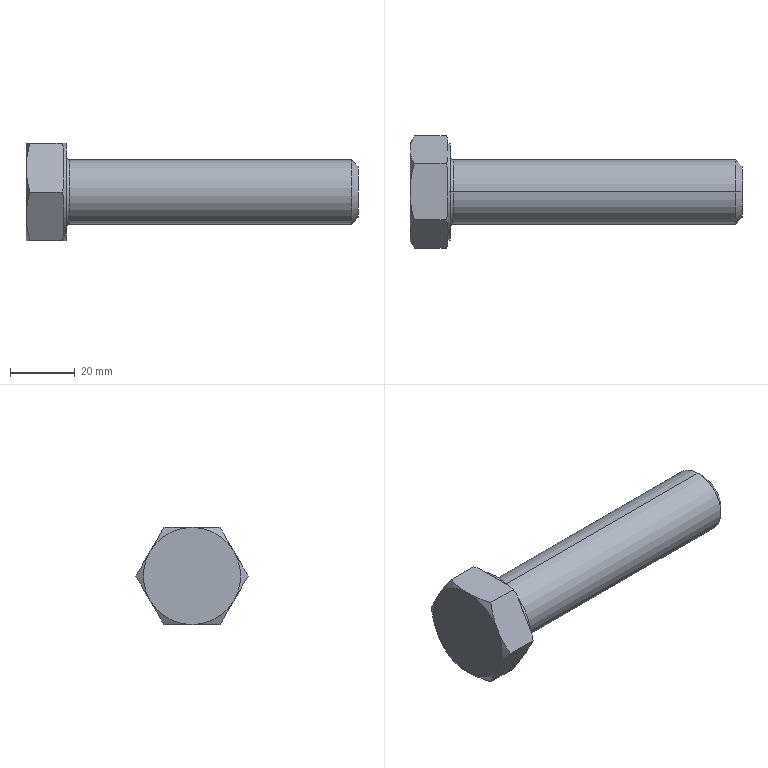Part | SolidWorks | features RevCut 4, Chamfer 1, Extrusion 1, Fillet 1, LPattern 1, Revolution 1 | 1 solid | 35 faces | box 102.5 x 34.641 x 30 mm | volume 37820 mm3 | plane 15 | cone 14 | cylinder 4 | torus 2 | commonest cylinder face diameters 20 x2 30 x2
STEP:
#1=CARTESIAN_POINT('',(13.3,0.,10.));
#2=VERTEX_POINT('',#1);
#3=CARTESIAN_POINT('',(13.3,0.,-10.));
#4=VERTEX_POINT('',#3);
#5=CARTESIAN_POINT('',(13.3,0.,0.));
#6=DIRECTION('',(1.,0.,0.));
#7=DIRECTION('',(0.,0.,-1.));
#8=AXIS2_PLACEMENT_3D('',#5,#6,#7);
#9=CIRCLE('',#8,10.);
#10=EDGE_CURVE('',#2,#4,#9,.T.);
#11=ORIENTED_EDGE('',*,*,#10,.F.);
#12=CARTESIAN_POINT('',(12.5,0.,10.8));
#13=VERTEX_POINT('',#12);
#14=CARTESIAN_POINT('',(13.3,0.,10.8));
#15=DIRECTION('',(0.,1.,0.));
#16=DIRECTION('',(0.,0.,1.));
#17=AXIS2_PLACEMENT_3D('',#14,#15,#16);
#18=CIRCLE('',#17,0.8);
#19=EDGE_CURVE('',#2,#13,#18,.T.);
#20=ORIENTED_EDGE('',*,*,#19,.T.);
#21=CARTESIAN_POINT('',(12.5,0.,-10.8));
#22=VERTEX_POINT('',#21);
#23=CARTESIAN_POINT('',(12.5,0.,0.));
#24=DIRECTION('',(-1.,0.,0.));
#25=DIRECTION('',(0.,0.,-1.));
#26=AXIS2_PLACEMENT_3D('',#23,#24,#25);
#27=CIRCLE('',#26,10.8);
#28=EDGE_CURVE('',#22,#13,#27,.T.);
#29=ORIENTED_EDGE('',*,*,#28,.F.);
#30=CARTESIAN_POINT('',(13.3,0.,-10.8));
#31=DIRECTION('',(0.,-1.,0.));
#32=DIRECTION('',(0.,0.,-1.));
#33=AXIS2_PLACEMENT_3D('',#30,#31,#32);
#34=CIRCLE('',#33,0.8);
#35=EDGE_CURVE('',#4,#22,#34,.T.);
#36=ORIENTED_EDGE('',*,*,#35,.F.);
#37=EDGE_LOOP('',(#11,#20,#29,#36));
#38=FACE_OUTER_BOUND('',#37,.T.);
#39=CARTESIAN_POINT('',(13.3,0.,0.));
#40=DIRECTION('',(1.,0.,0.));
#41=DIRECTION('',(0.,0.,-1.));
#42=AXIS2_PLACEMENT_3D('',#39,#40,#41);
#43=TOROIDAL_SURFACE('',#42,10.8,0.8);
#44=ADVANCED_FACE('',(#38),#43,.F.);
#45=CARTESIAN_POINT('',(102.5,0.,-8.));
#46=VERTEX_POINT('',#45);
#47=CARTESIAN_POINT('',(102.5,0.,8.));
#48=VERTEX_POINT('',#47);
#49=CARTESIAN_POINT('',(102.5,0.,0.));
#50=DIRECTION('',(1.,0.,0.));
#51=DIRECTION('',(0.,0.,1.));
#52=AXIS2_PLACEMENT_3D('',#49,#50,#51);
#53=CIRCLE('',#52,8.);
#54=EDGE_CURVE('',#46,#48,#53,.T.);
#55=ORIENTED_EDGE('',*,*,#54,.F.);
#56=CARTESIAN_POINT('',(100.5,0.,-10.));
#57=VERTEX_POINT('',#56);
#58=CARTESIAN_POINT('',(100.5,0.,-10.));
#59=DIRECTION('',(-0.7071,0.,-0.7071));
#60=VECTOR('',#59,1000.);
#61=LINE('',#58,#60);
#62=EDGE_CURVE('',#46,#57,#61,.T.);
#63=ORIENTED_EDGE('',*,*,#62,.T.);
#64=CARTESIAN_POINT('',(100.5,0.,10.));
#65=VERTEX_POINT('',#64);
#66=CARTESIAN_POINT('',(100.5,0.,0.));
#67=DIRECTION('',(-1.,0.,0.));
#68=DIRECTION('',(0.,0.,1.));
#69=AXIS2_PLACEMENT_3D('',#66,#67,#68);
#70=CIRCLE('',#69,10.);
#71=EDGE_CURVE('',#65,#57,#70,.T.);
#72=ORIENTED_EDGE('',*,*,#71,.F.);
#73=CARTESIAN_POINT('',(100.5,0.,10.));
#74=DIRECTION('',(-0.7071,0.,0.7071));
#75=VECTOR('',#74,1000.);
#76=LINE('',#73,#75);
#77=EDGE_CURVE('',#48,#65,#76,.T.);
#78=ORIENTED_EDGE('',*,*,#77,.F.);
#79=EDGE_LOOP('',(#55,#63,#72,#78));
#80=FACE_OUTER_BOUND('',#79,.T.);
#81=CARTESIAN_POINT('',(100.5,0.,0.));
#82=DIRECTION('',(-1.,0.,0.));
#83=DIRECTION('',(0.,0.,1.));
#84=AXIS2_PLACEMENT_3D('',#81,#82,#83);
#85=CONICAL_SURFACE('',#84,10.,0.7854);
#86=ADVANCED_FACE('',(#80),#85,.T.);
#87=ORIENTED_EDGE('',*,*,#71,.T.);
#88=CARTESIAN_POINT('',(0.,0.,-10.));
#89=DIRECTION('',(-1.,0.,0.));
#90=VECTOR('',#89,1000.);
#91=LINE('',#88,#90);
#92=EDGE_CURVE('',#57,#4,#91,.T.);
#93=ORIENTED_EDGE('',*,*,#92,.T.);
#94=CARTESIAN_POINT('',(13.3,0.,0.));
#95=DIRECTION('',(1.,0.,0.));
#96=DIRECTION('',(0.,0.,-1.));
#97=AXIS2_PLACEMENT_3D('',#94,#95,#96);
#98=CIRCLE('',#97,10.);
#99=EDGE_CURVE('',#4,#2,#98,.T.);
#100=ORIENTED_EDGE('',*,*,#99,.T.);
#101=CARTESIAN_POINT('',(0.,0.,10.));
#102=DIRECTION('',(-1.,0.,0.));
#103=VECTOR('',#102,1000.);
#104=LINE('',#101,#103);
#105=EDGE_CURVE('',#65,#2,#104,.T.);
#106=ORIENTED_EDGE('',*,*,#105,.F.);
#107=EDGE_LOOP('',(#87,#93,#100,#106));
#108=FACE_OUTER_BOUND('',#107,.T.);
#109=CARTESIAN_POINT('',(0.,0.,0.));
#110=DIRECTION('',(-1.,0.,0.));
#111=DIRECTION('',(0.,0.,1.));
#112=AXIS2_PLACEMENT_3D('',#109,#110,#111);
#113=CYLINDRICAL_SURFACE('',#112,10.);
#114=ADVANCED_FACE('',(#108),#113,.T.);
#115=CARTESIAN_POINT('',(12.5,0.,-15.));
#116=VERTEX_POINT('',#115);
#117=CARTESIAN_POINT('',(12.5,0.,15.));
#118=VERTEX_POINT('',#117);
#119=CARTESIAN_POINT('',(12.5,0.,0.));
#120=DIRECTION('',(1.,0.,0.));
#121=DIRECTION('',(0.,0.,-1.));
#122=AXIS2_PLACEMENT_3D('',#119,#120,#121);
#123=CIRCLE('',#122,15.);
#124=EDGE_CURVE('',#116,#118,#123,.T.);
#125=ORIENTED_EDGE('',*,*,#124,.F.);
#126=CARTESIAN_POINT('',(11.7,0.,-15.));
#127=VERTEX_POINT('',#126);
#128=CARTESIAN_POINT('',(0.,0.,-15.));
#129=DIRECTION('',(-1.,0.,0.));
#130=VECTOR('',#129,1000.);
#131=LINE('',#128,#130);
#132=EDGE_CURVE('',#116,#127,#131,.T.);
#133=ORIENTED_EDGE('',*,*,#132,.T.);
#134=CARTESIAN_POINT('',(11.7,12.99,-7.5));
#135=VERTEX_POINT('',#134);
#136=CARTESIAN_POINT('',(11.7,0.,0.));
#137=DIRECTION('',(-1.,0.,0.));
#138=DIRECTION('',(0.,0.,1.));
#139=AXIS2_PLACEMENT_3D('',#136,#137,#138);
#140=CIRCLE('',#139,15.);
#141=EDGE_CURVE('',#135,#127,#140,.T.);
#142=ORIENTED_EDGE('',*,*,#141,.F.);
#143=CARTESIAN_POINT('',(11.7,12.99,7.5));
#144=VERTEX_POINT('',#143);
#145=CARTESIAN_POINT('',(11.7,0.,0.));
#146=DIRECTION('',(-1.,0.,0.));
#147=DIRECTION('',(0.,0.,1.));
#148=AXIS2_PLACEMENT_3D('',#145,#146,#147);
#149=CIRCLE('',#148,15.);
#150=EDGE_CURVE('',#144,#135,#149,.T.);
#151=ORIENTED_EDGE('',*,*,#150,.F.);
#152=CARTESIAN_POINT('',(11.7,0.,15.));
#153=VERTEX_POINT('',#152);
#154=CARTESIAN_POINT('',(11.7,0.,0.));
#155=DIRECTION('',(-1.,0.,0.));
#156=DIRECTION('',(0.,0.,1.));
#157=AXIS2_PLACEMENT_3D('',#154,#155,#156);
#158=CIRCLE('',#157,15.);
#159=EDGE_CURVE('',#153,#144,#158,.T.);
#160=ORIENTED_EDGE('',*,*,#159,.F.);
#161=CARTESIAN_POINT('',(0.,0.,15.));
#162=DIRECTION('',(-1.,0.,0.));
#163=VECTOR('',#162,1000.);
#164=LINE('',#161,#163);
#165=EDGE_CURVE('',#118,#153,#164,.T.);
#166=ORIENTED_EDGE('',*,*,#165,.F.);
#167=EDGE_LOOP('',(#125,#133,#142,#151,#160,#166));
#168=FACE_OUTER_BOUND('',#167,.T.);
#169=CARTESIAN_POINT('',(0.,0.,0.));
#170=DIRECTION('',(-1.,0.,0.));
#171=DIRECTION('',(0.,0.,1.));
#172=AXIS2_PLACEMENT_3D('',#169,#170,#171);
#173=CYLINDRICAL_SURFACE('',#172,15.);
#174=ADVANCED_FACE('',(#168),#173,.T.);
#175=CARTESIAN_POINT('',(11.7,9.693,-13.211));
#176=VERTEX_POINT('',#175);
#177=CARTESIAN_POINT('',(11.7,8.66,-15.));
#178=DIRECTION('',(0.,0.5,0.866));
#179=VECTOR('',#178,1000.);
#180=LINE('',#177,#179);
#181=EDGE_CURVE('',#176,#135,#180,.T.);
#182=ORIENTED_EDGE('',*,*,#181,.F.);
#183=CARTESIAN_POINT('',(11.16,8.66,-15.));
#184=VERTEX_POINT('',#183);
#185=CARTESIAN_POINT('',(11.16,8.66,-15.));
#186=CARTESIAN_POINT('',(11.358,9.003,-14.406));
#187=CARTESIAN_POINT('',(11.539,9.347,-13.81));
#188=CARTESIAN_POINT('',(11.7,9.693,-13.211));
#189=B_SPLINE_CURVE_WITH_KNOTS('',3,(#185,#186,#187,#188),.UNSPECIFIED.,.F.,.F.,(4,4),(0.000000238,0.002122),.UNSPECIFIED.);
#190=EDGE_CURVE('',#184,#176,#189,.T.);
#191=ORIENTED_EDGE('',*,*,#190,.F.);
#192=CARTESIAN_POINT('',(1.34,8.66,-15.));
#193=VERTEX_POINT('',#192);
#194=CARTESIAN_POINT('',(12.5,8.66,-15.));
#195=DIRECTION('',(-1.,0.,0.));
#196=VECTOR('',#195,1000.);
#197=LINE('',#194,#196);
#198=EDGE_CURVE('',#184,#193,#197,.T.);
#199=ORIENTED_EDGE('',*,*,#198,.T.);
#200=CARTESIAN_POINT('',(0.,12.99,-7.5));
#201=VERTEX_POINT('',#200);
#202=CARTESIAN_POINT('',(0.,12.99,-7.5));
#203=CARTESIAN_POINT('',(0.,12.623,-8.136));
#204=CARTESIAN_POINT('',(0.03167,12.254,-8.776));
#205=CARTESIAN_POINT('',(0.1542,11.524,-10.041));
#206=CARTESIAN_POINT('',(0.245,11.161,-10.669));
#207=CARTESIAN_POINT('',(0.595,10.079,-12.542));
#208=CARTESIAN_POINT('',(0.9318,9.367,-13.776));
#209=CARTESIAN_POINT('',(1.34,8.66,-15.));
#210=B_SPLINE_CURVE_WITH_KNOTS('',3,(#202,#203,#204,#205,#206,#207,#208,#209),.UNSPECIFIED.,.F.,.F.,(4,2,2,4),(0.008763,0.01095,0.01313,0.01749),.UNSPECIFIED.);
#211=EDGE_CURVE('',#201,#193,#210,.T.);
#212=ORIENTED_EDGE('',*,*,#211,.F.);
#213=CARTESIAN_POINT('',(1.34,17.321,0.));
#214=VERTEX_POINT('',#213);
#215=CARTESIAN_POINT('',(1.34,17.321,0.));
#216=CARTESIAN_POINT('',(0.9308,16.612,-1.227));
#217=CARTESIAN_POINT('',(0.5939,15.899,-2.463));
#218=CARTESIAN_POINT('',(0.1277,14.457,-4.96));
#219=CARTESIAN_POINT('',(0.,13.728,-6.222));
#220=CARTESIAN_POINT('',(0.,12.99,-7.5));
#221=B_SPLINE_CURVE_WITH_KNOTS('',3,(#215,#216,#217,#218,#219,#220),.UNSPECIFIED.,.F.,.F.,(4,2,4),(0.000000238,0.004382,0.008763),.UNSPECIFIED.);
#222=EDGE_CURVE('',#214,#201,#221,.T.);
#223=ORIENTED_EDGE('',*,*,#222,.F.);
#224=CARTESIAN_POINT('',(11.16,17.321,0.));
#225=VERTEX_POINT('',#224);
#226=CARTESIAN_POINT('',(12.5,17.321,0.));
#227=DIRECTION('',(-1.,0.,0.));
#228=VECTOR('',#227,1000.);
#229=LINE('',#226,#228);
#230=EDGE_CURVE('',#225,#214,#229,.T.);
#231=ORIENTED_EDGE('',*,*,#230,.F.);
#232=CARTESIAN_POINT('',(11.7,16.288,-1.789));
#233=VERTEX_POINT('',#232);
#234=CARTESIAN_POINT('',(11.7,16.288,-1.789));
#235=CARTESIAN_POINT('',(11.539,16.634,-1.19));
#236=CARTESIAN_POINT('',(11.358,16.978,-0.5937));
#237=CARTESIAN_POINT('',(11.16,17.321,0.));
#238=B_SPLINE_CURVE_WITH_KNOTS('',3,(#234,#235,#236,#237),.UNSPECIFIED.,.F.,.F.,(4,4),(0.01538,0.01749),.UNSPECIFIED.);
#239=EDGE_CURVE('',#233,#225,#238,.T.);
#240=ORIENTED_EDGE('',*,*,#239,.F.);
#241=CARTESIAN_POINT('',(11.7,8.66,-15.));
#242=DIRECTION('',(0.,0.5,0.866));
#243=VECTOR('',#242,1000.);
#244=LINE('',#241,#243);
#245=EDGE_CURVE('',#135,#233,#244,.T.);
#246=ORIENTED_EDGE('',*,*,#245,.F.);
#247=EDGE_LOOP('',(#182,#191,#199,#212,#223,#231,#240,#246));
#248=FACE_OUTER_BOUND('',#247,.T.);
#249=CARTESIAN_POINT('',(12.5,8.66,-15.));
#250=DIRECTION('',(0.,-0.866,0.5));
#251=DIRECTION('',(0.,-0.5,-0.866));
#252=AXIS2_PLACEMENT_3D('',#249,#250,#251);
#253=PLANE('',#252);
#254=ADVANCED_FACE('',(#248),#253,.F.);
#255=CARTESIAN_POINT('',(11.7,16.288,1.789));
#256=VERTEX_POINT('',#255);
#257=CARTESIAN_POINT('',(11.7,17.321,0.));
#258=DIRECTION('',(0.,-0.5,0.866));
#259=VECTOR('',#258,1000.);
#260=LINE('',#257,#259);
#261=EDGE_CURVE('',#256,#144,#260,.T.);
#262=ORIENTED_EDGE('',*,*,#261,.F.);
#263=CARTESIAN_POINT('',(11.16,17.321,0.));
#264=CARTESIAN_POINT('',(11.358,16.978,0.594));
#265=CARTESIAN_POINT('',(11.539,16.633,1.19));
#266=CARTESIAN_POINT('',(11.7,16.288,1.789));
#267=B_SPLINE_CURVE_WITH_KNOTS('',3,(#263,#264,#265,#266),.UNSPECIFIED.,.F.,.F.,(4,4),(0.000000238,0.002122),.UNSPECIFIED.);
#268=EDGE_CURVE('',#225,#256,#267,.T.);
#269=ORIENTED_EDGE('',*,*,#268,.F.);
#270=ORIENTED_EDGE('',*,*,#230,.T.);
#271=CARTESIAN_POINT('',(0.,12.99,7.5));
#272=VERTEX_POINT('',#271);
#273=CARTESIAN_POINT('',(0.,12.99,7.5));
#274=CARTESIAN_POINT('',(0.,13.358,6.864));
#275=CARTESIAN_POINT('',(0.03167,13.727,6.224));
#276=CARTESIAN_POINT('',(0.1542,14.457,4.959));
#277=CARTESIAN_POINT('',(0.245,14.82,4.331));
#278=CARTESIAN_POINT('',(0.595,15.901,2.458));
#279=CARTESIAN_POINT('',(0.9318,16.614,1.224));
#280=CARTESIAN_POINT('',(1.34,17.321,0.));
#281=B_SPLINE_CURVE_WITH_KNOTS('',3,(#273,#274,#275,#276,#277,#278,#279,#280),.UNSPECIFIED.,.F.,.F.,(4,2,2,4),(0.008763,0.01095,0.01313,0.01749),.UNSPECIFIED.);
#282=EDGE_CURVE('',#272,#214,#281,.T.);
#283=ORIENTED_EDGE('',*,*,#282,.F.);
#284=CARTESIAN_POINT('',(1.34,8.66,15.));
#285=VERTEX_POINT('',#284);
#286=CARTESIAN_POINT('',(1.34,8.66,15.));
#287=CARTESIAN_POINT('',(0.9308,9.369,13.773));
#288=CARTESIAN_POINT('',(0.5939,10.082,12.537));
#289=CARTESIAN_POINT('',(0.1277,11.524,10.04));
#290=CARTESIAN_POINT('',(0.,12.253,8.778));
#291=CARTESIAN_POINT('',(0.,12.99,7.5));
#292=B_SPLINE_CURVE_WITH_KNOTS('',3,(#286,#287,#288,#289,#290,#291),.UNSPECIFIED.,.F.,.F.,(4,2,4),(0.000000238,0.004382,0.008763),.UNSPECIFIED.);
#293=EDGE_CURVE('',#285,#272,#292,.T.);
#294=ORIENTED_EDGE('',*,*,#293,.F.);
#295=CARTESIAN_POINT('',(11.16,8.66,15.));
#296=VERTEX_POINT('',#295);
#297=CARTESIAN_POINT('',(12.5,8.66,15.));
#298=DIRECTION('',(-1.,0.,0.));
#299=VECTOR('',#298,1000.);
#300=LINE('',#297,#299);
#301=EDGE_CURVE('',#296,#285,#300,.T.);
#302=ORIENTED_EDGE('',*,*,#301,.F.);
#303=CARTESIAN_POINT('',(11.7,9.693,13.211));
#304=VERTEX_POINT('',#303);
#305=CARTESIAN_POINT('',(11.7,9.693,13.211));
#306=CARTESIAN_POINT('',(11.539,9.347,13.81));
#307=CARTESIAN_POINT('',(11.358,9.003,14.406));
#308=CARTESIAN_POINT('',(11.16,8.66,15.));
#309=B_SPLINE_CURVE_WITH_KNOTS('',3,(#305,#306,#307,#308),.UNSPECIFIED.,.F.,.F.,(4,4),(0.01538,0.01749),.UNSPECIFIED.);
#310=EDGE_CURVE('',#304,#296,#309,.T.);
#311=ORIENTED_EDGE('',*,*,#310,.F.);
#312=CARTESIAN_POINT('',(11.7,17.321,0.));
#313=DIRECTION('',(0.,-0.5,0.866));
#314=VECTOR('',#313,1000.);
#315=LINE('',#312,#314);
#316=EDGE_CURVE('',#144,#304,#315,.T.);
#317=ORIENTED_EDGE('',*,*,#316,.F.);
#318=EDGE_LOOP('',(#262,#269,#270,#283,#294,#302,#311,#317));
#319=FACE_OUTER_BOUND('',#318,.T.);
#320=CARTESIAN_POINT('',(12.5,17.321,0.));
#321=DIRECTION('',(0.,-0.866,-0.5));
#322=DIRECTION('',(0.,0.5,-0.866));
#323=AXIS2_PLACEMENT_3D('',#320,#321,#322);
#324=PLANE('',#323);
#325=ADVANCED_FACE('',(#319),#324,.F.);
#326=CARTESIAN_POINT('',(11.7,6.595,15.));
#327=VERTEX_POINT('',#326);
#328=CARTESIAN_POINT('',(11.7,8.66,15.));
#329=DIRECTION('',(0.,-1.,0.));
#330=VECTOR('',#329,1000.);
#331=LINE('',#328,#330);
#332=EDGE_CURVE('',#327,#153,#331,.T.);
#333=ORIENTED_EDGE('',*,*,#332,.F.);
#334=CARTESIAN_POINT('',(11.16,8.66,15.));
#335=CARTESIAN_POINT('',(11.358,7.976,15.));
#336=CARTESIAN_POINT('',(11.539,7.288,15.));
#337=CARTESIAN_POINT('',(11.7,6.595,15.));
#338=B_SPLINE_CURVE_WITH_KNOTS('',3,(#334,#335,#336,#337),.UNSPECIFIED.,.F.,.F.,(4,4),(0.03969,0.04183),.UNSPECIFIED.);
#339=EDGE_CURVE('',#296,#327,#338,.T.);
#340=ORIENTED_EDGE('',*,*,#339,.F.);
#341=ORIENTED_EDGE('',*,*,#301,.T.);
#342=CARTESIAN_POINT('',(0.,0.,15.));
#343=VERTEX_POINT('',#342);
#344=CARTESIAN_POINT('',(0.,0.,15.));
#345=CARTESIAN_POINT('',(0.,0.7329,15.));
#346=CARTESIAN_POINT('',(0.03126,1.469,15.));
#347=CARTESIAN_POINT('',(0.1552,2.944,15.));
#348=CARTESIAN_POINT('',(0.2469,3.673,15.));
#349=CARTESIAN_POINT('',(0.5989,5.841,15.));
#350=CARTESIAN_POINT('',(0.9354,7.26,15.));
#351=CARTESIAN_POINT('',(1.34,8.66,15.));
#352=B_SPLINE_CURVE_WITH_KNOTS('',3,(#344,#345,#346,#347,#348,#349,#350,#351),.UNSPECIFIED.,.F.,.F.,(4,2,2,4),(0.02466,0.02686,0.02905,0.03344),.UNSPECIFIED.);
#353=EDGE_CURVE('',#343,#285,#352,.T.);
#354=ORIENTED_EDGE('',*,*,#353,.F.);
#355=CARTESIAN_POINT('',(1.34,-8.66,15.));
#356=VERTEX_POINT('',#355);
#357=CARTESIAN_POINT('',(1.34,-8.66,15.));
#358=CARTESIAN_POINT('',(0.9328,-7.25,15.));
#359=CARTESIAN_POINT('',(0.592,-5.808,15.));
#360=CARTESIAN_POINT('',(0.126,-2.919,15.));
#361=CARTESIAN_POINT('',(0.,-1.465,15.));
#362=CARTESIAN_POINT('',(0.,0.,15.));
#363=B_SPLINE_CURVE_WITH_KNOTS('',3,(#357,#358,#359,#360,#361,#362),.UNSPECIFIED.,.F.,.F.,(4,2,4),(0.0159,0.02028,0.02466),.UNSPECIFIED.);
#364=EDGE_CURVE('',#356,#343,#363,.T.);
#365=ORIENTED_EDGE('',*,*,#364,.F.);
#366=CARTESIAN_POINT('',(11.16,-8.66,15.));
#367=VERTEX_POINT('',#366);
#368=CARTESIAN_POINT('',(12.5,-8.66,15.));
#369=DIRECTION('',(-1.,0.,0.));
#370=VECTOR('',#369,1000.);
#371=LINE('',#368,#370);
#372=EDGE_CURVE('',#367,#356,#371,.T.);
#373=ORIENTED_EDGE('',*,*,#372,.F.);
#374=CARTESIAN_POINT('',(11.7,-6.595,15.));
#375=VERTEX_POINT('',#374);
#376=CARTESIAN_POINT('',(11.7,-6.595,15.));
#377=CARTESIAN_POINT('',(11.539,-7.289,15.));
#378=CARTESIAN_POINT('',(11.357,-7.978,15.));
#379=CARTESIAN_POINT('',(11.16,-8.66,15.));
#380=B_SPLINE_CURVE_WITH_KNOTS('',3,(#376,#377,#378,#379),.UNSPECIFIED.,.F.,.F.,(4,4),(0.05511,0.05723),.UNSPECIFIED.);
#381=EDGE_CURVE('',#375,#367,#380,.T.);
#382=ORIENTED_EDGE('',*,*,#381,.F.);
#383=CARTESIAN_POINT('',(11.7,8.66,15.));
#384=DIRECTION('',(0.,-1.,0.));
#385=VECTOR('',#384,1000.);
#386=LINE('',#383,#385);
#387=EDGE_CURVE('',#153,#375,#386,.T.);
#388=ORIENTED_EDGE('',*,*,#387,.F.);
#389=EDGE_LOOP('',(#333,#340,#341,#354,#365,#373,#382,#388));
#390=FACE_OUTER_BOUND('',#389,.T.);
#391=CARTESIAN_POINT('',(12.5,8.66,15.));
#392=DIRECTION('',(0.,0.,-1.));
#393=DIRECTION('',(-1.,0.,0.));
#394=AXIS2_PLACEMENT_3D('',#391,#392,#393);
#395=PLANE('',#394);
#396=ADVANCED_FACE('',(#390),#395,.F.);
#397=CARTESIAN_POINT('',(11.7,-9.693,13.211));
#398=VERTEX_POINT('',#397);
#399=CARTESIAN_POINT('',(11.7,-12.99,7.5));
#400=VERTEX_POINT('',#399);
#401=CARTESIAN_POINT('',(11.7,-17.321,0.));
#402=DIRECTION('',(0.,-0.5,-0.866));
#403=VECTOR('',#402,1000.);
#404=LINE('',#401,#403);
#405=EDGE_CURVE('',#398,#400,#404,.T.);
#406=ORIENTED_EDGE('',*,*,#405,.F.);
#407=CARTESIAN_POINT('',(11.16,-8.66,15.));
#408=CARTESIAN_POINT('',(11.358,-9.003,14.406));
#409=CARTESIAN_POINT('',(11.539,-9.347,13.81));
#410=CARTESIAN_POINT('',(11.7,-9.693,13.211));
#411=B_SPLINE_CURVE_WITH_KNOTS('',3,(#407,#408,#409,#410),.UNSPECIFIED.,.F.,.F.,(4,4),(0.000000238,0.002122),.UNSPECIFIED.);
#412=EDGE_CURVE('',#367,#398,#411,.T.);
#413=ORIENTED_EDGE('',*,*,#412,.F.);
#414=ORIENTED_EDGE('',*,*,#372,.T.);
#415=CARTESIAN_POINT('',(0.,-12.99,7.5));
#416=VERTEX_POINT('',#415);
#417=CARTESIAN_POINT('',(0.,-12.99,7.5));
#418=CARTESIAN_POINT('',(0.,-12.623,8.136));
#419=CARTESIAN_POINT('',(0.03167,-12.254,8.776));
#420=CARTESIAN_POINT('',(0.1542,-11.524,10.041));
#421=CARTESIAN_POINT('',(0.245,-11.161,10.669));
#422=CARTESIAN_POINT('',(0.595,-10.079,12.542));
#423=CARTESIAN_POINT('',(0.9318,-9.367,13.776));
#424=CARTESIAN_POINT('',(1.34,-8.66,15.));
#425=B_SPLINE_CURVE_WITH_KNOTS('',3,(#417,#418,#419,#420,#421,#422,#423,#424),.UNSPECIFIED.,.F.,.F.,(4,2,2,4),(0.008763,0.01095,0.01313,0.01749),.UNSPECIFIED.);
#426=EDGE_CURVE('',#416,#356,#425,.T.);
#427=ORIENTED_EDGE('',*,*,#426,.F.);
#428=CARTESIAN_POINT('',(1.34,-17.321,0.));
#429=VERTEX_POINT('',#428);
#430=CARTESIAN_POINT('',(1.34,-17.321,0.));
#431=CARTESIAN_POINT('',(0.9308,-16.612,1.227));
#432=CARTESIAN_POINT('',(0.5939,-15.899,2.463));
#433=CARTESIAN_POINT('',(0.1277,-14.457,4.96));
#434=CARTESIAN_POINT('',(0.,-13.728,6.222));
#435=CARTESIAN_POINT('',(0.,-12.99,7.5));
#436=B_SPLINE_CURVE_WITH_KNOTS('',3,(#430,#431,#432,#433,#434,#435),.UNSPECIFIED.,.F.,.F.,(4,2,4),(0.000000238,0.004382,0.008763),.UNSPECIFIED.);
#437=EDGE_CURVE('',#429,#416,#436,.T.);
#438=ORIENTED_EDGE('',*,*,#437,.F.);
#439=CARTESIAN_POINT('',(11.16,-17.321,0.));
#440=VERTEX_POINT('',#439);
#441=CARTESIAN_POINT('',(12.5,-17.321,0.));
#442=DIRECTION('',(-1.,0.,0.));
#443=VECTOR('',#442,1000.);
#444=LINE('',#441,#443);
#445=EDGE_CURVE('',#440,#429,#444,.T.);
#446=ORIENTED_EDGE('',*,*,#445,.F.);
#447=CARTESIAN_POINT('',(11.7,-16.288,1.789));
#448=VERTEX_POINT('',#447);
#449=CARTESIAN_POINT('',(11.7,-16.288,1.789));
#450=CARTESIAN_POINT('',(11.539,-16.634,1.19));
#451=CARTESIAN_POINT('',(11.358,-16.978,0.5937));
#452=CARTESIAN_POINT('',(11.16,-17.321,0.));
#453=B_SPLINE_CURVE_WITH_KNOTS('',3,(#449,#450,#451,#452),.UNSPECIFIED.,.F.,.F.,(4,4),(0.01538,0.01749),.UNSPECIFIED.);
#454=EDGE_CURVE('',#448,#440,#453,.T.);
#455=ORIENTED_EDGE('',*,*,#454,.F.);
#456=CARTESIAN_POINT('',(11.7,-17.321,0.));
#457=DIRECTION('',(0.,-0.5,-0.866));
#458=VECTOR('',#457,1000.);
#459=LINE('',#456,#458);
#460=EDGE_CURVE('',#400,#448,#459,.T.);
#461=ORIENTED_EDGE('',*,*,#460,.F.);
#462=EDGE_LOOP('',(#406,#413,#414,#427,#438,#446,#455,#461));
#463=FACE_OUTER_BOUND('',#462,.T.);
#464=CARTESIAN_POINT('',(12.5,-17.321,0.));
#465=DIRECTION('',(0.,0.866,-0.5));
#466=DIRECTION('',(0.,0.5,0.866));
#467=AXIS2_PLACEMENT_3D('',#464,#465,#466);
#468=PLANE('',#467);
#469=ADVANCED_FACE('',(#463),#468,.F.);
#470=CARTESIAN_POINT('',(11.7,-16.288,-1.789));
#471=VERTEX_POINT('',#470);
#472=CARTESIAN_POINT('',(11.7,-12.99,-7.5));
#473=VERTEX_POINT('',#472);
#474=CARTESIAN_POINT('',(11.7,-8.66,-15.));
#475=DIRECTION('',(0.,0.5,-0.866));
#476=VECTOR('',#475,1000.);
#477=LINE('',#474,#476);
#478=EDGE_CURVE('',#471,#473,#477,.T.);
#479=ORIENTED_EDGE('',*,*,#478,.F.);
#480=CARTESIAN_POINT('',(11.16,-17.321,0.));
#481=CARTESIAN_POINT('',(11.358,-16.978,-0.594));
#482=CARTESIAN_POINT('',(11.539,-16.633,-1.19));
#483=CARTESIAN_POINT('',(11.7,-16.288,-1.789));
#484=B_SPLINE_CURVE_WITH_KNOTS('',3,(#480,#481,#482,#483),.UNSPECIFIED.,.F.,.F.,(4,4),(0.000000238,0.002122),.UNSPECIFIED.);
#485=EDGE_CURVE('',#440,#471,#484,.T.);
#486=ORIENTED_EDGE('',*,*,#485,.F.);
#487=ORIENTED_EDGE('',*,*,#445,.T.);
#488=CARTESIAN_POINT('',(0.,-12.99,-7.5));
#489=VERTEX_POINT('',#488);
#490=CARTESIAN_POINT('',(0.,-12.99,-7.5));
#491=CARTESIAN_POINT('',(0.,-13.358,-6.864));
#492=CARTESIAN_POINT('',(0.03167,-13.727,-6.224));
#493=CARTESIAN_POINT('',(0.1542,-14.457,-4.959));
#494=CARTESIAN_POINT('',(0.245,-14.82,-4.331));
#495=CARTESIAN_POINT('',(0.595,-15.901,-2.458));
#496=CARTESIAN_POINT('',(0.9318,-16.614,-1.224));
#497=CARTESIAN_POINT('',(1.34,-17.321,0.));
#498=B_SPLINE_CURVE_WITH_KNOTS('',3,(#490,#491,#492,#493,#494,#495,#496,#497),.UNSPECIFIED.,.F.,.F.,(4,2,2,4),(0.008763,0.01095,0.01313,0.01749),.UNSPECIFIED.);
#499=EDGE_CURVE('',#489,#429,#498,.T.);
#500=ORIENTED_EDGE('',*,*,#499,.F.);
#501=CARTESIAN_POINT('',(1.34,-8.66,-15.));
#502=VERTEX_POINT('',#501);
#503=CARTESIAN_POINT('',(1.34,-8.66,-15.));
#504=CARTESIAN_POINT('',(0.9308,-9.369,-13.773));
#505=CARTESIAN_POINT('',(0.5939,-10.082,-12.537));
#506=CARTESIAN_POINT('',(0.1277,-11.524,-10.04));
#507=CARTESIAN_POINT('',(0.,-12.253,-8.778));
#508=CARTESIAN_POINT('',(0.,-12.99,-7.5));
#509=B_SPLINE_CURVE_WITH_KNOTS('',3,(#503,#504,#505,#506,#507,#508),.UNSPECIFIED.,.F.,.F.,(4,2,4),(0.000000238,0.004382,0.008763),.UNSPECIFIED.);
#510=EDGE_CURVE('',#502,#489,#509,.T.);
#511=ORIENTED_EDGE('',*,*,#510,.F.);
#512=CARTESIAN_POINT('',(11.16,-8.66,-15.));
#513=VERTEX_POINT('',#512);
#514=CARTESIAN_POINT('',(12.5,-8.66,-15.));
#515=DIRECTION('',(-1.,0.,0.));
#516=VECTOR('',#515,1000.);
#517=LINE('',#514,#516);
#518=EDGE_CURVE('',#513,#502,#517,.T.);
#519=ORIENTED_EDGE('',*,*,#518,.F.);
#520=CARTESIAN_POINT('',(11.7,-9.693,-13.211));
#521=VERTEX_POINT('',#520);
#522=CARTESIAN_POINT('',(11.7,-9.693,-13.211));
#523=CARTESIAN_POINT('',(11.539,-9.347,-13.81));
#524=CARTESIAN_POINT('',(11.358,-9.003,-14.406));
#525=CARTESIAN_POINT('',(11.16,-8.66,-15.));
#526=B_SPLINE_CURVE_WITH_KNOTS('',3,(#522,#523,#524,#525),.UNSPECIFIED.,.F.,.F.,(4,4),(0.01538,0.01749),.UNSPECIFIED.);
#527=EDGE_CURVE('',#521,#513,#526,.T.);
#528=ORIENTED_EDGE('',*,*,#527,.F.);
#529=CARTESIAN_POINT('',(11.7,-8.66,-15.));
#530=DIRECTION('',(0.,0.5,-0.866));
#531=VECTOR('',#530,1000.);
#532=LINE('',#529,#531);
#533=EDGE_CURVE('',#473,#521,#532,.T.);
#534=ORIENTED_EDGE('',*,*,#533,.F.);
#535=EDGE_LOOP('',(#479,#486,#487,#500,#511,#519,#528,#534));
#536=FACE_OUTER_BOUND('',#535,.T.);
#537=CARTESIAN_POINT('',(12.5,-8.66,-15.));
#538=DIRECTION('',(0.,0.866,0.5));
#539=DIRECTION('',(0.,-0.5,0.866));
#540=AXIS2_PLACEMENT_3D('',#537,#538,#539);
#541=PLANE('',#540);
#542=ADVANCED_FACE('',(#536),#541,.F.);
#543=CARTESIAN_POINT('',(11.7,-6.595,-15.));
#544=VERTEX_POINT('',#543);
#545=CARTESIAN_POINT('',(11.7,8.66,-15.));
#546=DIRECTION('',(0.,1.,0.));
#547=VECTOR('',#546,1000.);
#548=LINE('',#545,#547);
#549=EDGE_CURVE('',#544,#127,#548,.T.);
#550=ORIENTED_EDGE('',*,*,#549,.F.);
#551=CARTESIAN_POINT('',(11.16,-8.66,-15.));
#552=CARTESIAN_POINT('',(11.357,-7.978,-15.));
#553=CARTESIAN_POINT('',(11.539,-7.289,-15.));
#554=CARTESIAN_POINT('',(11.7,-6.595,-15.));
#555=B_SPLINE_CURVE_WITH_KNOTS('',3,(#551,#552,#553,#554),.UNSPECIFIED.,.F.,.F.,(4,4),(0.0159,0.01802),.UNSPECIFIED.);
#556=EDGE_CURVE('',#513,#544,#555,.T.);
#557=ORIENTED_EDGE('',*,*,#556,.F.);
#558=ORIENTED_EDGE('',*,*,#518,.T.);
#559=CARTESIAN_POINT('',(0.,0.,-15.));
#560=VERTEX_POINT('',#559);
#561=CARTESIAN_POINT('',(0.,0.,-15.));
#562=CARTESIAN_POINT('',(0.,-1.465,-15.));
#563=CARTESIAN_POINT('',(0.126,-2.919,-15.));
#564=CARTESIAN_POINT('',(0.592,-5.808,-15.));
#565=CARTESIAN_POINT('',(0.9328,-7.25,-15.));
#566=CARTESIAN_POINT('',(1.34,-8.66,-15.));
#567=B_SPLINE_CURVE_WITH_KNOTS('',3,(#561,#562,#563,#564,#565,#566),.UNSPECIFIED.,.F.,.F.,(4,2,4),(0.04846,0.05285,0.05723),.UNSPECIFIED.);
#568=EDGE_CURVE('',#560,#502,#567,.T.);
#569=ORIENTED_EDGE('',*,*,#568,.F.);
#570=CARTESIAN_POINT('',(1.34,8.66,-15.));
#571=CARTESIAN_POINT('',(0.9354,7.26,-15.));
#572=CARTESIAN_POINT('',(0.5989,5.841,-15.));
#573=CARTESIAN_POINT('',(0.2469,3.673,-15.));
#574=CARTESIAN_POINT('',(0.1552,2.944,-15.));
#575=CARTESIAN_POINT('',(0.03126,1.469,-15.));
#576=CARTESIAN_POINT('',(0.,0.7329,-15.));
#577=CARTESIAN_POINT('',(0.,0.,-15.));
#578=B_SPLINE_CURVE_WITH_KNOTS('',3,(#570,#571,#572,#573,#574,#575,#576,#577),.UNSPECIFIED.,.F.,.F.,(4,2,2,4),(0.03969,0.04407,0.04627,0.04846),.UNSPECIFIED.);
#579=EDGE_CURVE('',#193,#560,#578,.T.);
#580=ORIENTED_EDGE('',*,*,#579,.F.);
#581=ORIENTED_EDGE('',*,*,#198,.F.);
#582=CARTESIAN_POINT('',(11.7,6.595,-15.));
#583=VERTEX_POINT('',#582);
#584=CARTESIAN_POINT('',(11.7,6.595,-15.));
#585=CARTESIAN_POINT('',(11.539,7.288,-15.));
#586=CARTESIAN_POINT('',(11.358,7.976,-15.));
#587=CARTESIAN_POINT('',(11.16,8.66,-15.));
#588=B_SPLINE_CURVE_WITH_KNOTS('',3,(#584,#585,#586,#587),.UNSPECIFIED.,.F.,.F.,(4,4),(0.03129,0.03344),.UNSPECIFIED.);
#589=EDGE_CURVE('',#583,#184,#588,.T.);
#590=ORIENTED_EDGE('',*,*,#589,.F.);
#591=CARTESIAN_POINT('',(11.7,8.66,-15.));
#592=DIRECTION('',(0.,1.,0.));
#593=VECTOR('',#592,1000.);
#594=LINE('',#591,#593);
#595=EDGE_CURVE('',#127,#583,#594,.T.);
#596=ORIENTED_EDGE('',*,*,#595,.F.);
#597=EDGE_LOOP('',(#550,#557,#558,#569,#580,#581,#590,#596));
#598=FACE_OUTER_BOUND('',#597,.T.);
#599=CARTESIAN_POINT('',(12.5,8.66,-15.));
#600=DIRECTION('',(0.,0.,1.));
#601=DIRECTION('',(1.,0.,0.));
#602=AXIS2_PLACEMENT_3D('',#599,#600,#601);
#603=PLANE('',#602);
#604=ADVANCED_FACE('',(#598),#603,.F.);
#605=ORIENTED_EDGE('',*,*,#556,.T.);
#606=CARTESIAN_POINT('',(11.7,0.,0.));
#607=DIRECTION('',(-1.,0.,0.));
#608=DIRECTION('',(0.,0.,-1.));
#609=AXIS2_PLACEMENT_3D('',#606,#607,#608);
#610=CIRCLE('',#609,16.386);
#611=EDGE_CURVE('',#544,#521,#610,.T.);
#612=ORIENTED_EDGE('',*,*,#611,.T.);
#613=ORIENTED_EDGE('',*,*,#527,.T.);
#614=EDGE_LOOP('',(#605,#612,#613));
#615=FACE_OUTER_BOUND('',#614,.T.);
#616=CARTESIAN_POINT('',(8.274,0.,0.));
#617=DIRECTION('',(-1.,0.,0.));
#618=DIRECTION('',(0.,0.,1.));
#619=AXIS2_PLACEMENT_3D('',#616,#617,#618);
#620=CONICAL_SURFACE('',#619,22.321,1.047);
#621=ADVANCED_FACE('',(#615),#620,.T.);
#622=ORIENTED_EDGE('',*,*,#485,.T.);
#623=CARTESIAN_POINT('',(11.7,0.,0.));
#624=DIRECTION('',(-1.,0.,0.));
#625=DIRECTION('',(0.,0.,-1.));
#626=AXIS2_PLACEMENT_3D('',#623,#624,#625);
#627=CIRCLE('',#626,16.386);
#628=EDGE_CURVE('',#471,#448,#627,.T.);
#629=ORIENTED_EDGE('',*,*,#628,.T.);
#630=ORIENTED_EDGE('',*,*,#454,.T.);
#631=EDGE_LOOP('',(#622,#629,#630));
#632=FACE_OUTER_BOUND('',#631,.T.);
#633=CARTESIAN_POINT('',(8.274,0.,0.));
#634=DIRECTION('',(-1.,0.,0.));
#635=DIRECTION('',(0.,0.,1.));
#636=AXIS2_PLACEMENT_3D('',#633,#634,#635);
#637=CONICAL_SURFACE('',#636,22.321,1.047);
#638=ADVANCED_FACE('',(#632),#637,.T.);
#639=ORIENTED_EDGE('',*,*,#412,.T.);
#640=CARTESIAN_POINT('',(11.7,0.,0.));
#641=DIRECTION('',(-1.,0.,0.));
#642=DIRECTION('',(0.,0.,-1.));
#643=AXIS2_PLACEMENT_3D('',#640,#641,#642);
#644=CIRCLE('',#643,16.386);
#645=EDGE_CURVE('',#398,#375,#644,.T.);
#646=ORIENTED_EDGE('',*,*,#645,.T.);
#647=ORIENTED_EDGE('',*,*,#381,.T.);
#648=EDGE_LOOP('',(#639,#646,#647));
#649=FACE_OUTER_BOUND('',#648,.T.);
#650=CARTESIAN_POINT('',(8.274,0.,0.));
#651=DIRECTION('',(-1.,0.,0.));
#652=DIRECTION('',(0.,0.,1.));
#653=AXIS2_PLACEMENT_3D('',#650,#651,#652);
#654=CONICAL_SURFACE('',#653,22.321,1.047);
#655=ADVANCED_FACE('',(#649),#654,.T.);
#656=ORIENTED_EDGE('',*,*,#339,.T.);
#657=CARTESIAN_POINT('',(11.7,0.,0.));
#658=DIRECTION('',(-1.,0.,0.));
#659=DIRECTION('',(0.,0.,-1.));
#660=AXIS2_PLACEMENT_3D('',#657,#658,#659);
#661=CIRCLE('',#660,16.386);
#662=EDGE_CURVE('',#327,#304,#661,.T.);
#663=ORIENTED_EDGE('',*,*,#662,.T.);
#664=ORIENTED_EDGE('',*,*,#310,.T.);
#665=EDGE_LOOP('',(#656,#663,#664));
#666=FACE_OUTER_BOUND('',#665,.T.);
#667=CARTESIAN_POINT('',(8.274,0.,0.));
#668=DIRECTION('',(-1.,0.,0.));
#669=DIRECTION('',(0.,0.,1.));
#670=AXIS2_PLACEMENT_3D('',#667,#668,#669);
#671=CONICAL_SURFACE('',#670,22.321,1.047);
#672=ADVANCED_FACE('',(#666),#671,.T.);
#673=ORIENTED_EDGE('',*,*,#268,.T.);
#674=CARTESIAN_POINT('',(11.7,0.,0.));
#675=DIRECTION('',(-1.,0.,0.));
#676=DIRECTION('',(0.,0.,-1.));
#677=AXIS2_PLACEMENT_3D('',#674,#675,#676);
#678=CIRCLE('',#677,16.386);
#679=EDGE_CURVE('',#256,#233,#678,.T.);
#680=ORIENTED_EDGE('',*,*,#679,.T.);
#681=ORIENTED_EDGE('',*,*,#239,.T.);
#682=EDGE_LOOP('',(#673,#680,#681));
#683=FACE_OUTER_BOUND('',#682,.T.);
#684=CARTESIAN_POINT('',(8.274,0.,0.));
#685=DIRECTION('',(-1.,0.,0.));
#686=DIRECTION('',(0.,0.,1.));
#687=AXIS2_PLACEMENT_3D('',#684,#685,#686);
#688=CONICAL_SURFACE('',#687,22.321,1.047);
#689=ADVANCED_FACE('',(#683),#688,.T.);
#690=ORIENTED_EDGE('',*,*,#190,.T.);
#691=CARTESIAN_POINT('',(11.7,0.,0.));
#692=DIRECTION('',(-1.,0.,0.));
#693=DIRECTION('',(0.,0.,-1.));
#694=AXIS2_PLACEMENT_3D('',#691,#692,#693);
#695=CIRCLE('',#694,16.386);
#696=EDGE_CURVE('',#176,#583,#695,.T.);
#697=ORIENTED_EDGE('',*,*,#696,.T.);
#698=ORIENTED_EDGE('',*,*,#589,.T.);
#699=EDGE_LOOP('',(#690,#697,#698));
#700=FACE_OUTER_BOUND('',#699,.T.);
#701=CARTESIAN_POINT('',(8.274,0.,0.));
#702=DIRECTION('',(-1.,0.,0.));
#703=DIRECTION('',(0.,0.,1.));
#704=AXIS2_PLACEMENT_3D('',#701,#702,#703);
#705=CONICAL_SURFACE('',#704,22.321,1.047);
#706=ADVANCED_FACE('',(#700),#705,.T.);
#707=ORIENTED_EDGE('',*,*,#510,.T.);
#708=CARTESIAN_POINT('',(0.,0.,0.));
#709=DIRECTION('',(1.,0.,0.));
#710=DIRECTION('',(0.,0.,-1.));
#711=AXIS2_PLACEMENT_3D('',#708,#709,#710);
#712=CIRCLE('',#711,15.);
#713=EDGE_CURVE('',#489,#560,#712,.T.);
#714=ORIENTED_EDGE('',*,*,#713,.T.);
#715=ORIENTED_EDGE('',*,*,#568,.T.);
#716=EDGE_LOOP('',(#707,#714,#715));
#717=FACE_OUTER_BOUND('',#716,.T.);
#718=CARTESIAN_POINT('',(0.,0.,0.));
#719=DIRECTION('',(1.,0.,0.));
#720=DIRECTION('',(0.,0.,-1.));
#721=AXIS2_PLACEMENT_3D('',#718,#719,#720);
#722=CONICAL_SURFACE('',#721,15.,1.047);
#723=ADVANCED_FACE('',(#717),#722,.T.);
#724=ORIENTED_EDGE('',*,*,#437,.T.);
#725=CARTESIAN_POINT('',(0.,0.,0.));
#726=DIRECTION('',(1.,0.,0.));
#727=DIRECTION('',(0.,0.,-1.));
#728=AXIS2_PLACEMENT_3D('',#725,#726,#727);
#729=CIRCLE('',#728,15.);
#730=EDGE_CURVE('',#416,#489,#729,.T.);
#731=ORIENTED_EDGE('',*,*,#730,.T.);
#732=ORIENTED_EDGE('',*,*,#499,.T.);
#733=EDGE_LOOP('',(#724,#731,#732));
#734=FACE_OUTER_BOUND('',#733,.T.);
#735=CARTESIAN_POINT('',(0.,0.,0.));
#736=DIRECTION('',(1.,0.,0.));
#737=DIRECTION('',(0.,0.,-1.));
#738=AXIS2_PLACEMENT_3D('',#735,#736,#737);
#739=CONICAL_SURFACE('',#738,15.,1.047);
#740=ADVANCED_FACE('',(#734),#739,.T.);
#741=ORIENTED_EDGE('',*,*,#364,.T.);
#742=CARTESIAN_POINT('',(0.,0.,0.));
#743=DIRECTION('',(1.,0.,0.));
#744=DIRECTION('',(0.,0.,-1.));
#745=AXIS2_PLACEMENT_3D('',#742,#743,#744);
#746=CIRCLE('',#745,15.);
#747=EDGE_CURVE('',#343,#416,#746,.T.);
#748=ORIENTED_EDGE('',*,*,#747,.T.);
#749=ORIENTED_EDGE('',*,*,#426,.T.);
#750=EDGE_LOOP('',(#741,#748,#749));
#751=FACE_OUTER_BOUND('',#750,.T.);
#752=CARTESIAN_POINT('',(0.,0.,0.));
#753=DIRECTION('',(1.,0.,0.));
#754=DIRECTION('',(0.,0.,-1.));
#755=AXIS2_PLACEMENT_3D('',#752,#753,#754);
#756=CONICAL_SURFACE('',#755,15.,1.047);
#757=ADVANCED_FACE('',(#751),#756,.T.);
#758=ORIENTED_EDGE('',*,*,#353,.T.);
#759=ORIENTED_EDGE('',*,*,#293,.T.);
#760=CARTESIAN_POINT('',(0.,0.,0.));
#761=DIRECTION('',(-1.,0.,0.));
#762=DIRECTION('',(0.,0.,1.));
#763=AXIS2_PLACEMENT_3D('',#760,#761,#762);
#764=CIRCLE('',#763,15.);
#765=EDGE_CURVE('',#343,#272,#764,.T.);
#766=ORIENTED_EDGE('',*,*,#765,.F.);
#767=EDGE_LOOP('',(#758,#759,#766));
#768=FACE_OUTER_BOUND('',#767,.T.);
#769=CARTESIAN_POINT('',(0.,0.,0.));
#770=DIRECTION('',(1.,0.,0.));
#771=DIRECTION('',(0.,0.,-1.));
#772=AXIS2_PLACEMENT_3D('',#769,#770,#771);
#773=CONICAL_SURFACE('',#772,15.,1.047);
#774=ADVANCED_FACE('',(#768),#773,.T.);
#775=ORIENTED_EDGE('',*,*,#282,.T.);
#776=ORIENTED_EDGE('',*,*,#222,.T.);
#777=CARTESIAN_POINT('',(0.,0.,0.));
#778=DIRECTION('',(1.,0.,0.));
#779=DIRECTION('',(0.,0.,-1.));
#780=AXIS2_PLACEMENT_3D('',#777,#778,#779);
#781=CIRCLE('',#780,15.);
#782=EDGE_CURVE('',#201,#272,#781,.T.);
#783=ORIENTED_EDGE('',*,*,#782,.T.);
#784=EDGE_LOOP('',(#775,#776,#783));
#785=FACE_OUTER_BOUND('',#784,.T.);
#786=CARTESIAN_POINT('',(0.,0.,0.));
#787=DIRECTION('',(1.,0.,0.));
#788=DIRECTION('',(0.,0.,-1.));
#789=AXIS2_PLACEMENT_3D('',#786,#787,#788);
#790=CONICAL_SURFACE('',#789,15.,1.047);
#791=ADVANCED_FACE('',(#785),#790,.T.);
#792=ORIENTED_EDGE('',*,*,#211,.T.);
#793=ORIENTED_EDGE('',*,*,#579,.T.);
#794=CARTESIAN_POINT('',(0.,0.,0.));
#795=DIRECTION('',(1.,0.,0.));
#796=DIRECTION('',(0.,0.,-1.));
#797=AXIS2_PLACEMENT_3D('',#794,#795,#796);
#798=CIRCLE('',#797,15.);
#799=EDGE_CURVE('',#560,#201,#798,.T.);
#800=ORIENTED_EDGE('',*,*,#799,.T.);
#801=EDGE_LOOP('',(#792,#793,#800));
#802=FACE_OUTER_BOUND('',#801,.T.);
#803=CARTESIAN_POINT('',(0.,0.,0.));
#804=DIRECTION('',(1.,0.,0.));
#805=DIRECTION('',(0.,0.,-1.));
#806=AXIS2_PLACEMENT_3D('',#803,#804,#805);
#807=CONICAL_SURFACE('',#806,15.,1.047);
#808=ADVANCED_FACE('',(#802),#807,.T.);
#809=ORIENTED_EDGE('',*,*,#799,.F.);
#810=ORIENTED_EDGE('',*,*,#713,.F.);
#811=ORIENTED_EDGE('',*,*,#730,.F.);
#812=ORIENTED_EDGE('',*,*,#747,.F.);
#813=ORIENTED_EDGE('',*,*,#765,.T.);
#814=ORIENTED_EDGE('',*,*,#782,.F.);
#815=EDGE_LOOP('',(#809,#810,#811,#812,#813,#814));
#816=FACE_OUTER_BOUND('',#815,.T.);
#817=CARTESIAN_POINT('',(0.,17.321,0.));
#818=DIRECTION('',(1.,0.,0.));
#819=DIRECTION('',(0.,0.,-1.));
#820=AXIS2_PLACEMENT_3D('',#817,#818,#819);
#821=PLANE('',#820);
#822=ADVANCED_FACE('',(#816),#821,.F.);
#823=ORIENTED_EDGE('',*,*,#387,.T.);
#824=ORIENTED_EDGE('',*,*,#645,.F.);
#825=ORIENTED_EDGE('',*,*,#405,.T.);
#826=CARTESIAN_POINT('',(11.7,0.,0.));
#827=DIRECTION('',(-1.,0.,0.));
#828=DIRECTION('',(0.,0.,1.));
#829=AXIS2_PLACEMENT_3D('',#826,#827,#828);
#830=CIRCLE('',#829,15.);
#831=EDGE_CURVE('',#400,#153,#830,.T.);
#832=ORIENTED_EDGE('',*,*,#831,.T.);
#833=EDGE_LOOP('',(#823,#824,#825,#832));
#834=FACE_OUTER_BOUND('',#833,.T.);
#835=CARTESIAN_POINT('',(11.7,15.,0.));
#836=DIRECTION('',(1.,0.,0.));
#837=DIRECTION('',(0.,0.,-1.));
#838=AXIS2_PLACEMENT_3D('',#835,#836,#837);
#839=PLANE('',#838);
#840=ADVANCED_FACE('',(#834),#839,.T.);
#841=ORIENTED_EDGE('',*,*,#261,.T.);
#842=ORIENTED_EDGE('',*,*,#150,.T.);
#843=ORIENTED_EDGE('',*,*,#245,.T.);
#844=ORIENTED_EDGE('',*,*,#679,.F.);
#845=EDGE_LOOP('',(#841,#842,#843,#844));
#846=FACE_OUTER_BOUND('',#845,.T.);
#847=CARTESIAN_POINT('',(11.7,15.,0.));
#848=DIRECTION('',(1.,0.,0.));
#849=DIRECTION('',(0.,0.,-1.));
#850=AXIS2_PLACEMENT_3D('',#847,#848,#849);
#851=PLANE('',#850);
#852=ADVANCED_FACE('',(#846),#851,.T.);
#853=ORIENTED_EDGE('',*,*,#460,.T.);
#854=ORIENTED_EDGE('',*,*,#628,.F.);
#855=ORIENTED_EDGE('',*,*,#478,.T.);
#856=CARTESIAN_POINT('',(11.7,0.,0.));
#857=DIRECTION('',(-1.,0.,0.));
#858=DIRECTION('',(0.,0.,1.));
#859=AXIS2_PLACEMENT_3D('',#856,#857,#858);
#860=CIRCLE('',#859,15.);
#861=EDGE_CURVE('',#473,#400,#860,.T.);
#862=ORIENTED_EDGE('',*,*,#861,.T.);
#863=EDGE_LOOP('',(#853,#854,#855,#862));
#864=FACE_OUTER_BOUND('',#863,.T.);
#865=CARTESIAN_POINT('',(11.7,15.,0.));
#866=DIRECTION('',(1.,0.,0.));
#867=DIRECTION('',(0.,0.,-1.));
#868=AXIS2_PLACEMENT_3D('',#865,#866,#867);
#869=PLANE('',#868);
#870=ADVANCED_FACE('',(#864),#869,.T.);
#871=ORIENTED_EDGE('',*,*,#533,.T.);
#872=ORIENTED_EDGE('',*,*,#611,.F.);
#873=ORIENTED_EDGE('',*,*,#549,.T.);
#874=CARTESIAN_POINT('',(11.7,0.,0.));
#875=DIRECTION('',(-1.,0.,0.));
#876=DIRECTION('',(0.,0.,1.));
#877=AXIS2_PLACEMENT_3D('',#874,#875,#876);
#878=CIRCLE('',#877,15.);
#879=EDGE_CURVE('',#127,#473,#878,.T.);
#880=ORIENTED_EDGE('',*,*,#879,.T.);
#881=EDGE_LOOP('',(#871,#872,#873,#880));
#882=FACE_OUTER_BOUND('',#881,.T.);
#883=CARTESIAN_POINT('',(11.7,15.,0.));
#884=DIRECTION('',(1.,0.,0.));
#885=DIRECTION('',(0.,0.,-1.));
#886=AXIS2_PLACEMENT_3D('',#883,#884,#885);
#887=PLANE('',#886);
#888=ADVANCED_FACE('',(#882),#887,.T.);
#889=ORIENTED_EDGE('',*,*,#181,.T.);
#890=ORIENTED_EDGE('',*,*,#141,.T.);
#891=ORIENTED_EDGE('',*,*,#595,.T.);
#892=ORIENTED_EDGE('',*,*,#696,.F.);
#893=EDGE_LOOP('',(#889,#890,#891,#892));
#894=FACE_OUTER_BOUND('',#893,.T.);
#895=CARTESIAN_POINT('',(11.7,15.,0.));
#896=DIRECTION('',(1.,0.,0.));
#897=DIRECTION('',(0.,0.,-1.));
#898=AXIS2_PLACEMENT_3D('',#895,#896,#897);
#899=PLANE('',#898);
#900=ADVANCED_FACE('',(#894),#899,.T.);
#901=ORIENTED_EDGE('',*,*,#132,.F.);
#902=CARTESIAN_POINT('',(12.5,0.,0.));
#903=DIRECTION('',(1.,0.,0.));
#904=DIRECTION('',(0.,0.,-1.));
#905=AXIS2_PLACEMENT_3D('',#902,#903,#904);
#906=CIRCLE('',#905,15.);
#907=EDGE_CURVE('',#118,#116,#906,.T.);
#908=ORIENTED_EDGE('',*,*,#907,.F.);
#909=ORIENTED_EDGE('',*,*,#165,.T.);
#910=ORIENTED_EDGE('',*,*,#831,.F.);
#911=ORIENTED_EDGE('',*,*,#861,.F.);
#912=ORIENTED_EDGE('',*,*,#879,.F.);
#913=EDGE_LOOP('',(#901,#908,#909,#910,#911,#912));
#914=FACE_OUTER_BOUND('',#913,.T.);
#915=CARTESIAN_POINT('',(0.,0.,0.));
#916=DIRECTION('',(-1.,0.,0.));
#917=DIRECTION('',(0.,0.,1.));
#918=AXIS2_PLACEMENT_3D('',#915,#916,#917);
#919=CYLINDRICAL_SURFACE('',#918,15.);
#920=ADVANCED_FACE('',(#914),#919,.T.);
#921=ORIENTED_EDGE('',*,*,#332,.T.);
#922=ORIENTED_EDGE('',*,*,#159,.T.);
#923=ORIENTED_EDGE('',*,*,#316,.T.);
#924=ORIENTED_EDGE('',*,*,#662,.F.);
#925=EDGE_LOOP('',(#921,#922,#923,#924));
#926=FACE_OUTER_BOUND('',#925,.T.);
#927=CARTESIAN_POINT('',(11.7,15.,0.));
#928=DIRECTION('',(1.,0.,0.));
#929=DIRECTION('',(0.,0.,-1.));
#930=AXIS2_PLACEMENT_3D('',#927,#928,#929);
#931=PLANE('',#930);
#932=ADVANCED_FACE('',(#926),#931,.T.);
#933=CARTESIAN_POINT('',(102.5,0.,0.));
#934=DIRECTION('',(1.,0.,0.));
#935=DIRECTION('',(0.,0.,1.));
#936=AXIS2_PLACEMENT_3D('',#933,#934,#935);
#937=CIRCLE('',#936,8.);
#938=EDGE_CURVE('',#48,#46,#937,.T.);
#939=ORIENTED_EDGE('',*,*,#938,.T.);
#940=ORIENTED_EDGE('',*,*,#54,.T.);
#941=EDGE_LOOP('',(#939,#940));
#942=FACE_OUTER_BOUND('',#941,.T.);
#943=CARTESIAN_POINT('',(102.5,0.,0.));
#944=DIRECTION('',(-1.,0.,0.));
#945=DIRECTION('',(0.,0.,1.));
#946=AXIS2_PLACEMENT_3D('',#943,#944,#945);
#947=PLANE('',#946);
#948=ADVANCED_FACE('',(#942),#947,.F.);
#949=ORIENTED_EDGE('',*,*,#92,.F.);
#950=CARTESIAN_POINT('',(100.5,0.,0.));
#951=DIRECTION('',(-1.,0.,0.));
#952=DIRECTION('',(0.,0.,1.));
#953=AXIS2_PLACEMENT_3D('',#950,#951,#952);
#954=CIRCLE('',#953,10.);
#955=EDGE_CURVE('',#57,#65,#954,.T.);
#956=ORIENTED_EDGE('',*,*,#955,.T.);
#957=ORIENTED_EDGE('',*,*,#105,.T.);
#958=ORIENTED_EDGE('',*,*,#10,.T.);
#959=EDGE_LOOP('',(#949,#956,#957,#958));
#960=FACE_OUTER_BOUND('',#959,.T.);
#961=CARTESIAN_POINT('',(0.,0.,0.));
#962=DIRECTION('',(-1.,0.,0.));
#963=DIRECTION('',(0.,0.,1.));
#964=AXIS2_PLACEMENT_3D('',#961,#962,#963);
#965=CYLINDRICAL_SURFACE('',#964,10.);
#966=ADVANCED_FACE('',(#960),#965,.T.);
#967=ORIENTED_EDGE('',*,*,#28,.T.);
#968=CARTESIAN_POINT('',(12.5,0.,0.));
#969=DIRECTION('',(-1.,0.,0.));
#970=DIRECTION('',(0.,0.,-1.));
#971=AXIS2_PLACEMENT_3D('',#968,#969,#970);
#972=CIRCLE('',#971,10.8);
#973=EDGE_CURVE('',#13,#22,#972,.T.);
#974=ORIENTED_EDGE('',*,*,#973,.T.);
#975=EDGE_LOOP('',(#967,#974));
#976=FACE_BOUND('',#975,.T.);
#977=ORIENTED_EDGE('',*,*,#907,.T.);
#978=ORIENTED_EDGE('',*,*,#124,.T.);
#979=EDGE_LOOP('',(#977,#978));
#980=FACE_OUTER_BOUND('',#979,.T.);
#981=CARTESIAN_POINT('',(12.5,17.321,0.));
#982=DIRECTION('',(1.,0.,0.));
#983=DIRECTION('',(0.,0.,-1.));
#984=AXIS2_PLACEMENT_3D('',#981,#982,#983);
#985=PLANE('',#984);
#986=ADVANCED_FACE('',(#976,#980),#985,.T.);
#987=ORIENTED_EDGE('',*,*,#62,.F.);
#988=ORIENTED_EDGE('',*,*,#938,.F.);
#989=ORIENTED_EDGE('',*,*,#77,.T.);
#990=ORIENTED_EDGE('',*,*,#955,.F.);
#991=EDGE_LOOP('',(#987,#988,#989,#990));
#992=FACE_OUTER_BOUND('',#991,.T.);
#993=CARTESIAN_POINT('',(100.5,0.,0.));
#994=DIRECTION('',(-1.,0.,0.));
#995=DIRECTION('',(0.,0.,1.));
#996=AXIS2_PLACEMENT_3D('',#993,#994,#995);
#997=CONICAL_SURFACE('',#996,10.,0.7854);
#998=ADVANCED_FACE('',(#992),#997,.T.);
#999=ORIENTED_EDGE('',*,*,#19,.F.);
#1000=ORIENTED_EDGE('',*,*,#99,.F.);
#1001=ORIENTED_EDGE('',*,*,#35,.T.);
#1002=ORIENTED_EDGE('',*,*,#973,.F.);
#1003=EDGE_LOOP('',(#999,#1000,#1001,#1002));
#1004=FACE_OUTER_BOUND('',#1003,.T.);
#1005=CARTESIAN_POINT('',(13.3,0.,0.));
#1006=DIRECTION('',(1.,0.,0.));
#1007=DIRECTION('',(0.,0.,-1.));
#1008=AXIS2_PLACEMENT_3D('',#1005,#1006,#1007);
#1009=TOROIDAL_SURFACE('',#1008,10.8,0.8);
#1010=ADVANCED_FACE('',(#1004),#1009,.F.);
#1011=CLOSED_SHELL('',(#44,#86,#114,#174,#254,#325,#396,#469,#542,#604,#621,#638,#655,#672,#689,#706,#723,#740,#757,#774,#791,#808,#822,#840,#852,#870,#888,#900,#920,#932,#948,#966,#986,#998,#1010));
#1012=MANIFOLD_SOLID_BREP('',#1011);
#1013=CARTESIAN_POINT('',(0.,0.,0.));
#1014=DIRECTION('',(0.,0.,1.));
#1015=DIRECTION('',(1.,0.,0.));
#1016=AXIS2_PLACEMENT_3D('',#1013,#1014,#1015);
#1017=(LENGTH_UNIT()NAMED_UNIT(*)SI_UNIT(.MILLI.,.METRE.));
#1018=UNCERTAINTY_MEASURE_WITH_UNIT(LENGTH_MEASURE(0.00001),#1017,'','');
#1019=(NAMED_UNIT(*)PLANE_ANGLE_UNIT()SI_UNIT($,.RADIAN.));
#1020=(NAMED_UNIT(*)SI_UNIT($,.STERADIAN.)SOLID_ANGLE_UNIT());
#1021=(GEOMETRIC_REPRESENTATION_CONTEXT(3)GLOBAL_UNCERTAINTY_ASSIGNED_CONTEXT((#1018))GLOBAL_UNIT_ASSIGNED_CONTEXT((#1017,#1019,#1020))REPRESENTATION_CONTEXT('',''));
#1022=ADVANCED_BREP_SHAPE_REPRESENTATION('',(#1012,#1016),#1021);